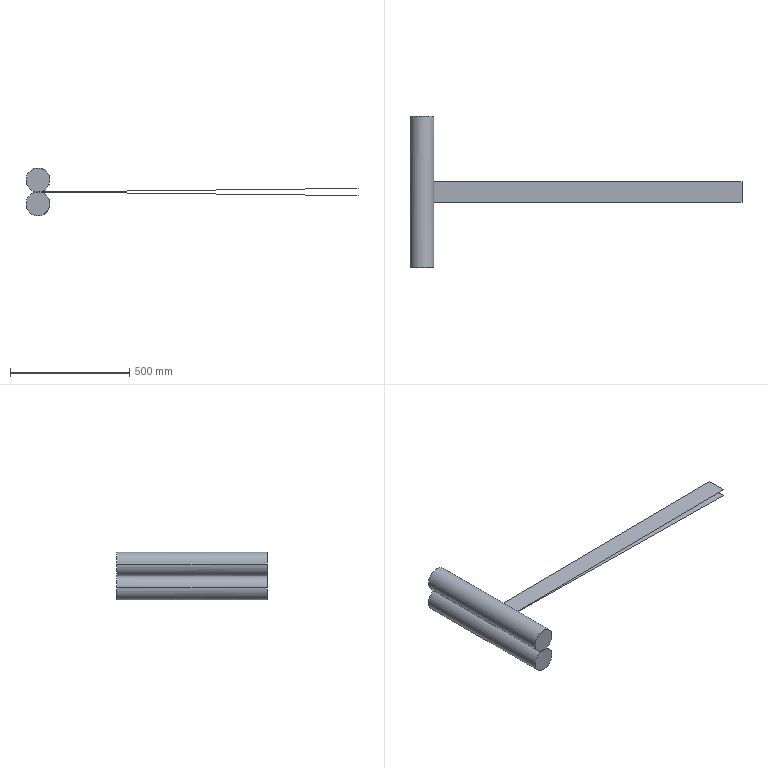Part | CATIA | 2 solids | 10 faces | box 1390 x 632 x 200 mm | volume 10069805 mm3 | plane 6 | cylinder 4 | commonest cylinder face diameters 100 x4